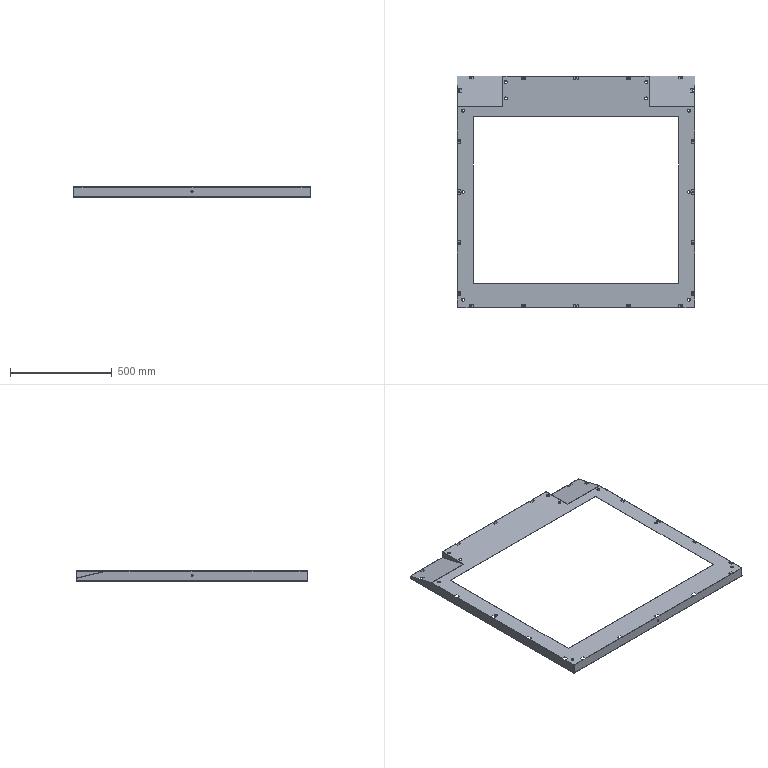Part | 3 solids | 402 faces | box 1169 x 1139 x 50 mm | volume 821282 mm3 | plane 258 | cylinder 128 | spline 16 | commonest cylinder face diameters 7 x50 0.4 x26 2.4 x26 14 x20 10 x6